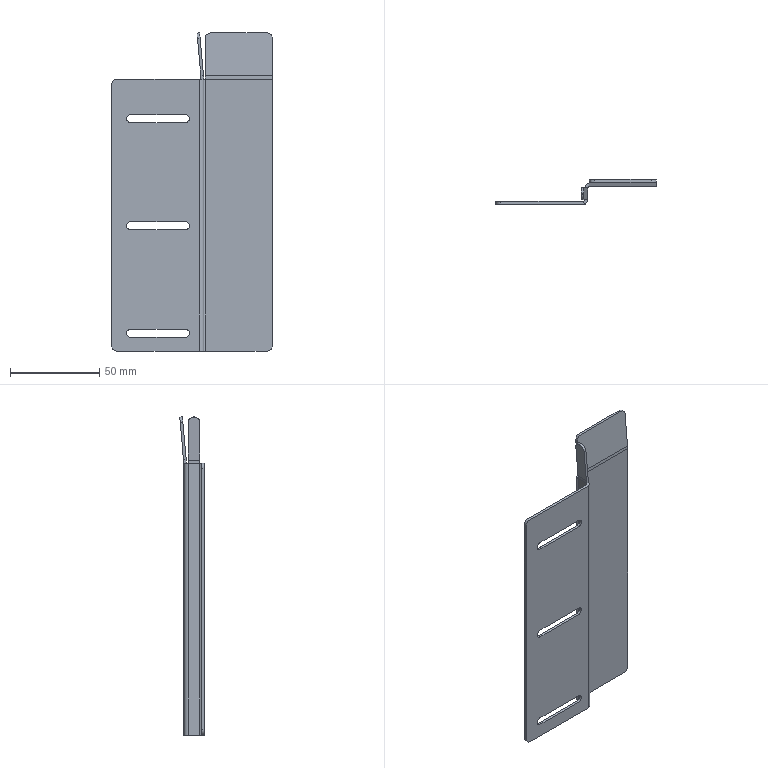Part | STEP file | 001-004-Feeding mechanism feed guide chute 1 | 1 solid | 69 faces | box 90 x 13.679 x 177.909 mm | volume 23460 mm3 | plane 42 | cylinder 21 | cone 6 | commonest cylinder face diameters 6 x7 4.5 x6 2 x2 5 x2 40 x2 43 x2